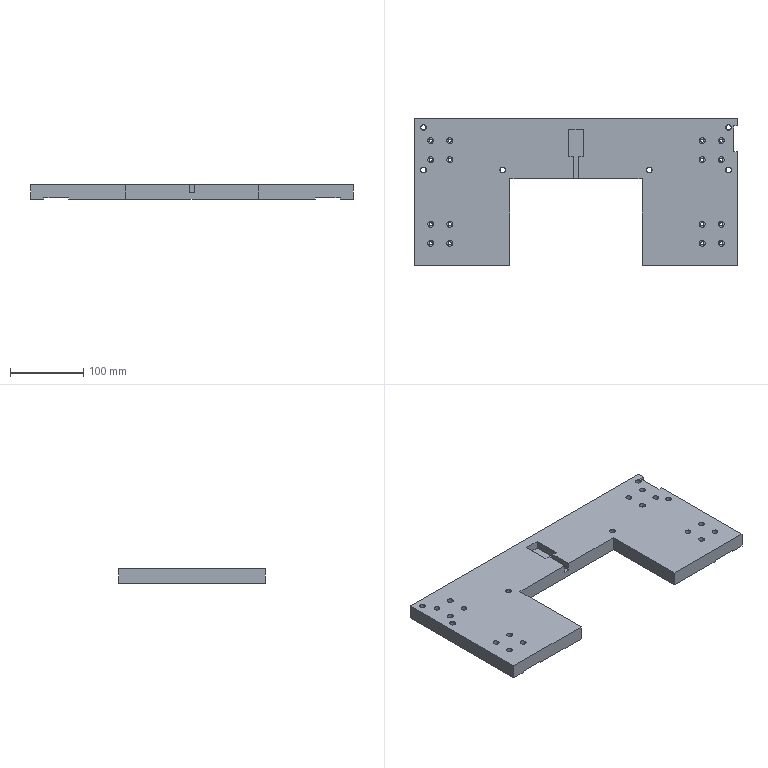Part | STEP file | Tube necking machine_id682_x_t | 1 solid | 102 faces | box 440 x 200 x 20 mm | volume 1280618 mm3 | plane 46 | cylinder 40 | cone 16 | commonest cylinder face diameters 4.5 x16 8 x16 6.8 x8